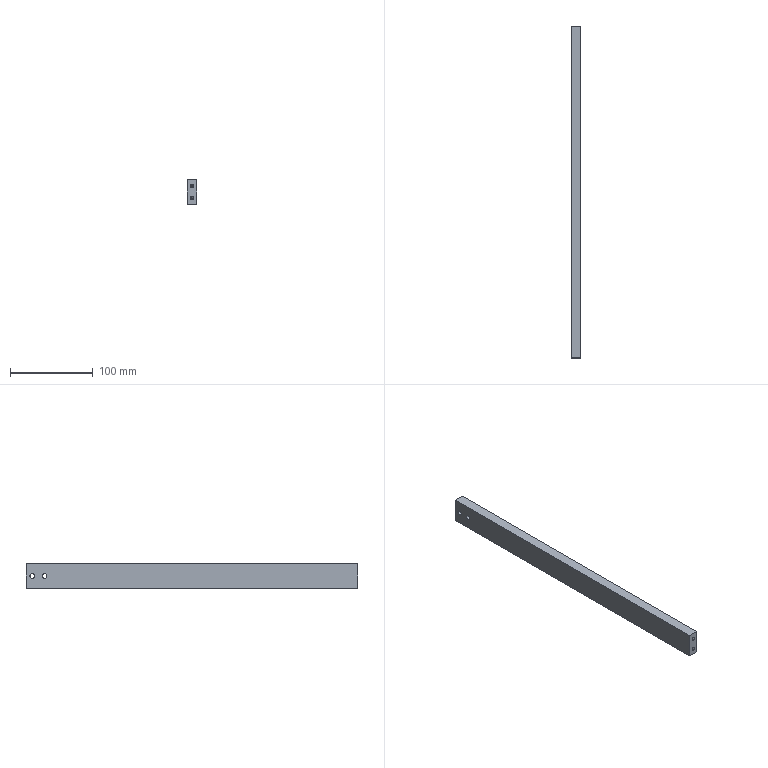Part | STEP file | 06-37 Heat-shrink tube support column | 1 solid | 24 faces | box 12 x 400 x 30 mm | volume 142471 mm3 | cylinder 12 | plane 8 | cone 4 | commonest cylinder face diameters 4.2 x4 5.5 x4 10 x4